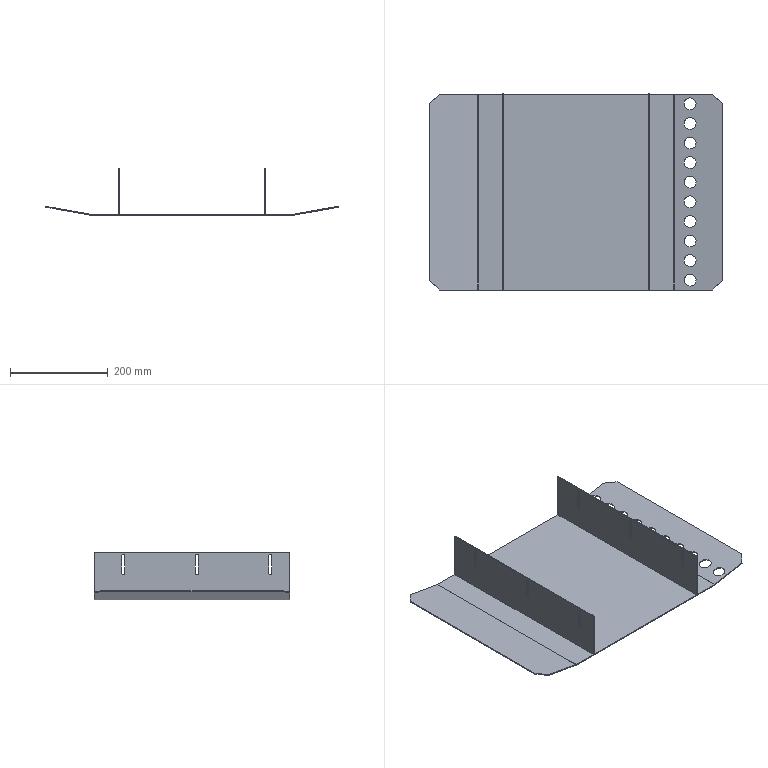Part | NX | 1 solid | 78 faces | box 597.656 x 400 x 97 mm | volume 618202 mm3 | plane 42 | spline 20 | cylinder 16 | commonest cylinder face diameters 6.5 x12 1.473 x2 5.473 x2